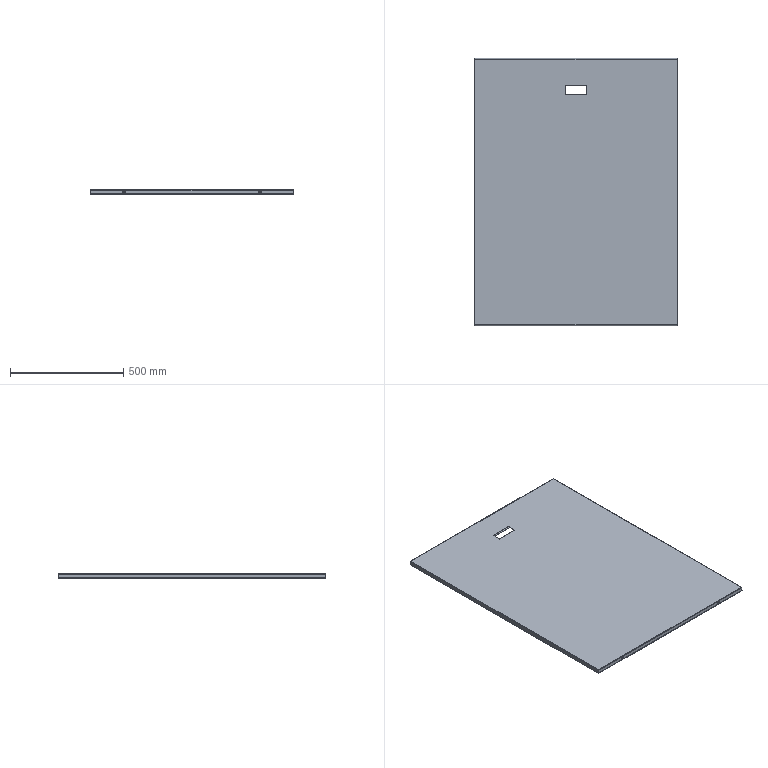Part | SolidWorks | features EdgeFlange 2, ICE 2, FlatPattern 1, SMBaseFlange 1, SheetMetal 1 | 1 solid | 78 faces | box 897 x 1178 x 20 mm | volume 1830546 mm3 | plane 42 | cylinder 20 | spline 16 | commonest cylinder face diameters 3 x8 5.4 x8 9 x4